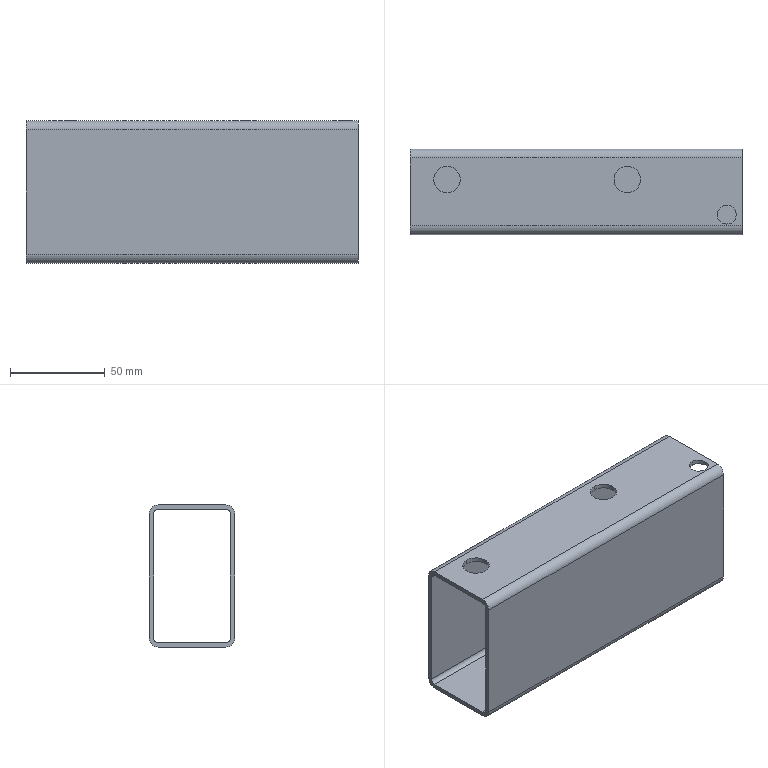Part | STEP file | [09] | 1 solid | 24 faces | box 175 x 45 x 75 mm | volume 89624 mm3 | cylinder 14 | plane 10 | commonest cylinder face diameters 4.6 x4 9.2 x4 14 x4 10 x2
STEP:
#1=CARTESIAN_POINT('',(167.,15.5,75.));
#2=VERTEX_POINT('',#1);
#3=CARTESIAN_POINT('',(167.,5.5,75.));
#4=VERTEX_POINT('',#3);
#5=CARTESIAN_POINT('',(167.,10.5,75.));
#6=DIRECTION('',(0.,0.,-1.));
#7=DIRECTION('',(0.,-1.,0.));
#8=AXIS2_PLACEMENT_3D('',#5,#6,#7);
#9=CIRCLE('',#8,5.);
#10=EDGE_CURVE('',#2,#4,#9,.T.);
#11=ORIENTED_EDGE('',*,*,#10,.F.);
#12=CARTESIAN_POINT('',(167.,15.5,72.7));
#13=VERTEX_POINT('',#12);
#14=CARTESIAN_POINT('',(167.,15.5,75.));
#15=DIRECTION('',(0.,0.,-1.));
#16=VECTOR('',#15,1000.);
#17=LINE('',#14,#16);
#18=EDGE_CURVE('',#2,#13,#17,.T.);
#19=ORIENTED_EDGE('',*,*,#18,.T.);
#20=CARTESIAN_POINT('',(167.,5.5,72.7));
#21=VERTEX_POINT('',#20);
#22=CARTESIAN_POINT('',(167.,10.5,72.7));
#23=DIRECTION('',(0.,0.,1.));
#24=DIRECTION('',(0.,1.,0.));
#25=AXIS2_PLACEMENT_3D('',#22,#23,#24);
#26=CIRCLE('',#25,5.);
#27=EDGE_CURVE('',#21,#13,#26,.T.);
#28=ORIENTED_EDGE('',*,*,#27,.F.);
#29=CARTESIAN_POINT('',(167.,5.5,75.));
#30=DIRECTION('',(0.,0.,-1.));
#31=VECTOR('',#30,1000.);
#32=LINE('',#29,#31);
#33=EDGE_CURVE('',#4,#21,#32,.T.);
#34=ORIENTED_EDGE('',*,*,#33,.F.);
#35=EDGE_LOOP('',(#11,#19,#28,#34));
#36=FACE_OUTER_BOUND('',#35,.T.);
#37=CARTESIAN_POINT('',(167.,10.5,75.));
#38=DIRECTION('',(0.,0.,-1.));
#39=DIRECTION('',(0.,-1.,0.));
#40=AXIS2_PLACEMENT_3D('',#37,#38,#39);
#41=CYLINDRICAL_SURFACE('',#40,5.);
#42=ADVANCED_FACE('',(#36),#41,.F.);
#43=CARTESIAN_POINT('',(114.5,36.,75.));
#44=VERTEX_POINT('',#43);
#45=CARTESIAN_POINT('',(114.5,22.,75.));
#46=VERTEX_POINT('',#45);
#47=CARTESIAN_POINT('',(114.5,29.,75.));
#48=DIRECTION('',(0.,0.,-1.));
#49=DIRECTION('',(0.,-1.,0.));
#50=AXIS2_PLACEMENT_3D('',#47,#48,#49);
#51=CIRCLE('',#50,7.);
#52=EDGE_CURVE('',#44,#46,#51,.T.);
#53=ORIENTED_EDGE('',*,*,#52,.F.);
#54=CARTESIAN_POINT('',(114.5,36.,72.7));
#55=VERTEX_POINT('',#54);
#56=CARTESIAN_POINT('',(114.5,36.,75.));
#57=DIRECTION('',(0.,0.,-1.));
#58=VECTOR('',#57,1000.);
#59=LINE('',#56,#58);
#60=EDGE_CURVE('',#44,#55,#59,.T.);
#61=ORIENTED_EDGE('',*,*,#60,.T.);
#62=CARTESIAN_POINT('',(114.5,22.,72.7));
#63=VERTEX_POINT('',#62);
#64=CARTESIAN_POINT('',(114.5,29.,72.7));
#65=DIRECTION('',(0.,0.,1.));
#66=DIRECTION('',(0.,1.,0.));
#67=AXIS2_PLACEMENT_3D('',#64,#65,#66);
#68=CIRCLE('',#67,7.);
#69=EDGE_CURVE('',#63,#55,#68,.T.);
#70=ORIENTED_EDGE('',*,*,#69,.F.);
#71=CARTESIAN_POINT('',(114.5,22.,75.));
#72=DIRECTION('',(0.,0.,-1.));
#73=VECTOR('',#72,1000.);
#74=LINE('',#71,#73);
#75=EDGE_CURVE('',#46,#63,#74,.T.);
#76=ORIENTED_EDGE('',*,*,#75,.F.);
#77=EDGE_LOOP('',(#53,#61,#70,#76));
#78=FACE_OUTER_BOUND('',#77,.T.);
#79=CARTESIAN_POINT('',(114.5,29.,75.));
#80=DIRECTION('',(0.,0.,-1.));
#81=DIRECTION('',(0.,-1.,0.));
#82=AXIS2_PLACEMENT_3D('',#79,#80,#81);
#83=CYLINDRICAL_SURFACE('',#82,7.);
#84=ADVANCED_FACE('',(#78),#83,.F.);
#85=CARTESIAN_POINT('',(19.5,36.,75.));
#86=VERTEX_POINT('',#85);
#87=CARTESIAN_POINT('',(19.5,22.,75.));
#88=VERTEX_POINT('',#87);
#89=CARTESIAN_POINT('',(19.5,29.,75.));
#90=DIRECTION('',(0.,0.,-1.));
#91=DIRECTION('',(0.,-1.,0.));
#92=AXIS2_PLACEMENT_3D('',#89,#90,#91);
#93=CIRCLE('',#92,7.);
#94=EDGE_CURVE('',#86,#88,#93,.T.);
#95=ORIENTED_EDGE('',*,*,#94,.F.);
#96=CARTESIAN_POINT('',(19.5,36.,72.7));
#97=VERTEX_POINT('',#96);
#98=CARTESIAN_POINT('',(19.5,36.,75.));
#99=DIRECTION('',(0.,0.,-1.));
#100=VECTOR('',#99,1000.);
#101=LINE('',#98,#100);
#102=EDGE_CURVE('',#86,#97,#101,.T.);
#103=ORIENTED_EDGE('',*,*,#102,.T.);
#104=CARTESIAN_POINT('',(19.5,22.,72.7));
#105=VERTEX_POINT('',#104);
#106=CARTESIAN_POINT('',(19.5,29.,72.7));
#107=DIRECTION('',(0.,0.,1.));
#108=DIRECTION('',(0.,1.,0.));
#109=AXIS2_PLACEMENT_3D('',#106,#107,#108);
#110=CIRCLE('',#109,7.);
#111=EDGE_CURVE('',#105,#97,#110,.T.);
#112=ORIENTED_EDGE('',*,*,#111,.F.);
#113=CARTESIAN_POINT('',(19.5,22.,75.));
#114=DIRECTION('',(0.,0.,-1.));
#115=VECTOR('',#114,1000.);
#116=LINE('',#113,#115);
#117=EDGE_CURVE('',#88,#105,#116,.T.);
#118=ORIENTED_EDGE('',*,*,#117,.F.);
#119=EDGE_LOOP('',(#95,#103,#112,#118));
#120=FACE_OUTER_BOUND('',#119,.T.);
#121=CARTESIAN_POINT('',(19.5,29.,75.));
#122=DIRECTION('',(0.,0.,-1.));
#123=DIRECTION('',(0.,-1.,0.));
#124=AXIS2_PLACEMENT_3D('',#121,#122,#123);
#125=CYLINDRICAL_SURFACE('',#124,7.);
#126=ADVANCED_FACE('',(#120),#125,.F.);
#127=CARTESIAN_POINT('',(0.,45.,70.4));
#128=VERTEX_POINT('',#127);
#129=CARTESIAN_POINT('',(0.,45.,4.6));
#130=VERTEX_POINT('',#129);
#131=CARTESIAN_POINT('',(0.,45.,70.4));
#132=DIRECTION('',(0.,0.,-1.));
#133=VECTOR('',#132,1000.);
#134=LINE('',#131,#133);
#135=EDGE_CURVE('',#128,#130,#134,.T.);
#136=ORIENTED_EDGE('',*,*,#135,.F.);
#137=CARTESIAN_POINT('',(175.,45.,70.4));
#138=VERTEX_POINT('',#137);
#139=CARTESIAN_POINT('',(175.,45.,70.4));
#140=DIRECTION('',(-1.,0.,0.));
#141=VECTOR('',#140,1000.);
#142=LINE('',#139,#141);
#143=EDGE_CURVE('',#138,#128,#142,.T.);
#144=ORIENTED_EDGE('',*,*,#143,.F.);
#145=CARTESIAN_POINT('',(175.,45.,4.6));
#146=VERTEX_POINT('',#145);
#147=CARTESIAN_POINT('',(175.,45.,70.4));
#148=DIRECTION('',(0.,0.,-1.));
#149=VECTOR('',#148,1000.);
#150=LINE('',#147,#149);
#151=EDGE_CURVE('',#138,#146,#150,.T.);
#152=ORIENTED_EDGE('',*,*,#151,.T.);
#153=CARTESIAN_POINT('',(175.,45.,4.6));
#154=DIRECTION('',(-1.,0.,0.));
#155=VECTOR('',#154,1000.);
#156=LINE('',#153,#155);
#157=EDGE_CURVE('',#146,#130,#156,.T.);
#158=ORIENTED_EDGE('',*,*,#157,.T.);
#159=EDGE_LOOP('',(#136,#144,#152,#158));
#160=FACE_OUTER_BOUND('',#159,.T.);
#161=CARTESIAN_POINT('',(175.,45.,70.4));
#162=DIRECTION('',(0.,1.,0.));
#163=DIRECTION('',(0.,0.,-1.));
#164=AXIS2_PLACEMENT_3D('',#161,#162,#163);
#165=PLANE('',#164);
#166=ADVANCED_FACE('',(#160),#165,.T.);
#167=CARTESIAN_POINT('',(0.,40.4,0.));
#168=VERTEX_POINT('',#167);
#169=CARTESIAN_POINT('',(0.,40.4,4.6));
#170=DIRECTION('',(-1.,0.,0.));
#171=DIRECTION('',(0.,1.,0.));
#172=AXIS2_PLACEMENT_3D('',#169,#170,#171);
#173=CIRCLE('',#172,4.6);
#174=EDGE_CURVE('',#130,#168,#173,.T.);
#175=ORIENTED_EDGE('',*,*,#174,.F.);
#176=ORIENTED_EDGE('',*,*,#157,.F.);
#177=CARTESIAN_POINT('',(175.,40.4,0.));
#178=VERTEX_POINT('',#177);
#179=CARTESIAN_POINT('',(175.,40.4,4.6));
#180=DIRECTION('',(-1.,0.,0.));
#181=DIRECTION('',(0.,1.,0.));
#182=AXIS2_PLACEMENT_3D('',#179,#180,#181);
#183=CIRCLE('',#182,4.6);
#184=EDGE_CURVE('',#146,#178,#183,.T.);
#185=ORIENTED_EDGE('',*,*,#184,.T.);
#186=CARTESIAN_POINT('',(175.,40.4,0.));
#187=DIRECTION('',(-1.,0.,0.));
#188=VECTOR('',#187,1000.);
#189=LINE('',#186,#188);
#190=EDGE_CURVE('',#178,#168,#189,.T.);
#191=ORIENTED_EDGE('',*,*,#190,.T.);
#192=EDGE_LOOP('',(#175,#176,#185,#191));
#193=FACE_OUTER_BOUND('',#192,.T.);
#194=CARTESIAN_POINT('',(175.,40.4,4.6));
#195=DIRECTION('',(-1.,0.,0.));
#196=DIRECTION('',(0.,1.,0.));
#197=AXIS2_PLACEMENT_3D('',#194,#195,#196);
#198=CYLINDRICAL_SURFACE('',#197,4.6);
#199=ADVANCED_FACE('',(#193),#198,.T.);
#200=CARTESIAN_POINT('',(0.,4.6,0.));
#201=VERTEX_POINT('',#200);
#202=CARTESIAN_POINT('',(0.,40.4,0.));
#203=DIRECTION('',(0.,-1.,0.));
#204=VECTOR('',#203,1000.);
#205=LINE('',#202,#204);
#206=EDGE_CURVE('',#168,#201,#205,.T.);
#207=ORIENTED_EDGE('',*,*,#206,.F.);
#208=ORIENTED_EDGE('',*,*,#190,.F.);
#209=CARTESIAN_POINT('',(175.,4.6,0.));
#210=VERTEX_POINT('',#209);
#211=CARTESIAN_POINT('',(175.,40.4,0.));
#212=DIRECTION('',(0.,-1.,0.));
#213=VECTOR('',#212,1000.);
#214=LINE('',#211,#213);
#215=EDGE_CURVE('',#178,#210,#214,.T.);
#216=ORIENTED_EDGE('',*,*,#215,.T.);
#217=CARTESIAN_POINT('',(175.,4.6,0.));
#218=DIRECTION('',(-1.,0.,0.));
#219=VECTOR('',#218,1000.);
#220=LINE('',#217,#219);
#221=EDGE_CURVE('',#210,#201,#220,.T.);
#222=ORIENTED_EDGE('',*,*,#221,.T.);
#223=EDGE_LOOP('',(#207,#208,#216,#222));
#224=FACE_OUTER_BOUND('',#223,.T.);
#225=CARTESIAN_POINT('',(175.,40.4,0.));
#226=DIRECTION('',(0.,0.,-1.));
#227=DIRECTION('',(0.,-1.,0.));
#228=AXIS2_PLACEMENT_3D('',#225,#226,#227);
#229=PLANE('',#228);
#230=ADVANCED_FACE('',(#224),#229,.T.);
#231=CARTESIAN_POINT('',(0.,0.,4.6));
#232=VERTEX_POINT('',#231);
#233=CARTESIAN_POINT('',(0.,4.6,4.6));
#234=DIRECTION('',(-1.,0.,0.));
#235=DIRECTION('',(0.,1.,0.));
#236=AXIS2_PLACEMENT_3D('',#233,#234,#235);
#237=CIRCLE('',#236,4.6);
#238=EDGE_CURVE('',#201,#232,#237,.T.);
#239=ORIENTED_EDGE('',*,*,#238,.F.);
#240=ORIENTED_EDGE('',*,*,#221,.F.);
#241=CARTESIAN_POINT('',(175.,0.,4.6));
#242=VERTEX_POINT('',#241);
#243=CARTESIAN_POINT('',(175.,4.6,4.6));
#244=DIRECTION('',(-1.,0.,0.));
#245=DIRECTION('',(0.,1.,0.));
#246=AXIS2_PLACEMENT_3D('',#243,#244,#245);
#247=CIRCLE('',#246,4.6);
#248=EDGE_CURVE('',#210,#242,#247,.T.);
#249=ORIENTED_EDGE('',*,*,#248,.T.);
#250=CARTESIAN_POINT('',(175.,0.,4.6));
#251=DIRECTION('',(-1.,0.,0.));
#252=VECTOR('',#251,1000.);
#253=LINE('',#250,#252);
#254=EDGE_CURVE('',#242,#232,#253,.T.);
#255=ORIENTED_EDGE('',*,*,#254,.T.);
#256=EDGE_LOOP('',(#239,#240,#249,#255));
#257=FACE_OUTER_BOUND('',#256,.T.);
#258=CARTESIAN_POINT('',(175.,4.6,4.6));
#259=DIRECTION('',(-1.,0.,0.));
#260=DIRECTION('',(0.,1.,0.));
#261=AXIS2_PLACEMENT_3D('',#258,#259,#260);
#262=CYLINDRICAL_SURFACE('',#261,4.6);
#263=ADVANCED_FACE('',(#257),#262,.T.);
#264=CARTESIAN_POINT('',(0.,0.,70.4));
#265=VERTEX_POINT('',#264);
#266=CARTESIAN_POINT('',(0.,0.,4.6));
#267=DIRECTION('',(0.,0.,1.));
#268=VECTOR('',#267,1000.);
#269=LINE('',#266,#268);
#270=EDGE_CURVE('',#232,#265,#269,.T.);
#271=ORIENTED_EDGE('',*,*,#270,.F.);
#272=ORIENTED_EDGE('',*,*,#254,.F.);
#273=CARTESIAN_POINT('',(175.,0.,70.4));
#274=VERTEX_POINT('',#273);
#275=CARTESIAN_POINT('',(175.,0.,4.6));
#276=DIRECTION('',(0.,0.,1.));
#277=VECTOR('',#276,1000.);
#278=LINE('',#275,#277);
#279=EDGE_CURVE('',#242,#274,#278,.T.);
#280=ORIENTED_EDGE('',*,*,#279,.T.);
#281=CARTESIAN_POINT('',(175.,0.,70.4));
#282=DIRECTION('',(-1.,0.,0.));
#283=VECTOR('',#282,1000.);
#284=LINE('',#281,#283);
#285=EDGE_CURVE('',#274,#265,#284,.T.);
#286=ORIENTED_EDGE('',*,*,#285,.T.);
#287=EDGE_LOOP('',(#271,#272,#280,#286));
#288=FACE_OUTER_BOUND('',#287,.T.);
#289=CARTESIAN_POINT('',(175.,0.,4.6));
#290=DIRECTION('',(0.,-1.,0.));
#291=DIRECTION('',(0.,0.,1.));
#292=AXIS2_PLACEMENT_3D('',#289,#290,#291);
#293=PLANE('',#292);
#294=ADVANCED_FACE('',(#288),#293,.T.);
#295=CARTESIAN_POINT('',(0.,4.6,75.));
#296=VERTEX_POINT('',#295);
#297=CARTESIAN_POINT('',(0.,4.6,70.4));
#298=DIRECTION('',(-1.,0.,0.));
#299=DIRECTION('',(0.,1.,0.));
#300=AXIS2_PLACEMENT_3D('',#297,#298,#299);
#301=CIRCLE('',#300,4.6);
#302=EDGE_CURVE('',#265,#296,#301,.T.);
#303=ORIENTED_EDGE('',*,*,#302,.F.);
#304=ORIENTED_EDGE('',*,*,#285,.F.);
#305=CARTESIAN_POINT('',(175.,4.6,75.));
#306=VERTEX_POINT('',#305);
#307=CARTESIAN_POINT('',(175.,4.6,70.4));
#308=DIRECTION('',(-1.,0.,0.));
#309=DIRECTION('',(0.,1.,0.));
#310=AXIS2_PLACEMENT_3D('',#307,#308,#309);
#311=CIRCLE('',#310,4.6);
#312=EDGE_CURVE('',#274,#306,#311,.T.);
#313=ORIENTED_EDGE('',*,*,#312,.T.);
#314=CARTESIAN_POINT('',(175.,4.6,75.));
#315=DIRECTION('',(-1.,0.,0.));
#316=VECTOR('',#315,1000.);
#317=LINE('',#314,#316);
#318=EDGE_CURVE('',#306,#296,#317,.T.);
#319=ORIENTED_EDGE('',*,*,#318,.T.);
#320=EDGE_LOOP('',(#303,#304,#313,#319));
#321=FACE_OUTER_BOUND('',#320,.T.);
#322=CARTESIAN_POINT('',(175.,4.6,70.4));
#323=DIRECTION('',(-1.,0.,0.));
#324=DIRECTION('',(0.,1.,0.));
#325=AXIS2_PLACEMENT_3D('',#322,#323,#324);
#326=CYLINDRICAL_SURFACE('',#325,4.6);
#327=ADVANCED_FACE('',(#321),#326,.T.);
#328=CARTESIAN_POINT('',(167.,10.5,75.));
#329=DIRECTION('',(0.,0.,-1.));
#330=DIRECTION('',(0.,-1.,0.));
#331=AXIS2_PLACEMENT_3D('',#328,#329,#330);
#332=CIRCLE('',#331,5.);
#333=EDGE_CURVE('',#4,#2,#332,.T.);
#334=ORIENTED_EDGE('',*,*,#333,.T.);
#335=ORIENTED_EDGE('',*,*,#10,.T.);
#336=EDGE_LOOP('',(#334,#335));
#337=FACE_BOUND('',#336,.T.);
#338=CARTESIAN_POINT('',(114.5,29.,75.));
#339=DIRECTION('',(0.,0.,-1.));
#340=DIRECTION('',(0.,-1.,0.));
#341=AXIS2_PLACEMENT_3D('',#338,#339,#340);
#342=CIRCLE('',#341,7.);
#343=EDGE_CURVE('',#46,#44,#342,.T.);
#344=ORIENTED_EDGE('',*,*,#343,.T.);
#345=ORIENTED_EDGE('',*,*,#52,.T.);
#346=EDGE_LOOP('',(#344,#345));
#347=FACE_BOUND('',#346,.T.);
#348=CARTESIAN_POINT('',(19.5,29.,75.));
#349=DIRECTION('',(0.,0.,-1.));
#350=DIRECTION('',(0.,-1.,0.));
#351=AXIS2_PLACEMENT_3D('',#348,#349,#350);
#352=CIRCLE('',#351,7.);
#353=EDGE_CURVE('',#88,#86,#352,.T.);
#354=ORIENTED_EDGE('',*,*,#353,.T.);
#355=ORIENTED_EDGE('',*,*,#94,.T.);
#356=EDGE_LOOP('',(#354,#355));
#357=FACE_BOUND('',#356,.T.);
#358=CARTESIAN_POINT('',(0.,40.4,75.));
#359=VERTEX_POINT('',#358);
#360=CARTESIAN_POINT('',(0.,4.6,75.));
#361=DIRECTION('',(0.,1.,0.));
#362=VECTOR('',#361,1000.);
#363=LINE('',#360,#362);
#364=EDGE_CURVE('',#296,#359,#363,.T.);
#365=ORIENTED_EDGE('',*,*,#364,.F.);
#366=ORIENTED_EDGE('',*,*,#318,.F.);
#367=CARTESIAN_POINT('',(175.,40.4,75.));
#368=VERTEX_POINT('',#367);
#369=CARTESIAN_POINT('',(175.,4.6,75.));
#370=DIRECTION('',(0.,1.,0.));
#371=VECTOR('',#370,1000.);
#372=LINE('',#369,#371);
#373=EDGE_CURVE('',#306,#368,#372,.T.);
#374=ORIENTED_EDGE('',*,*,#373,.T.);
#375=CARTESIAN_POINT('',(175.,40.4,75.));
#376=DIRECTION('',(-1.,0.,0.));
#377=VECTOR('',#376,1000.);
#378=LINE('',#375,#377);
#379=EDGE_CURVE('',#368,#359,#378,.T.);
#380=ORIENTED_EDGE('',*,*,#379,.T.);
#381=EDGE_LOOP('',(#365,#366,#374,#380));
#382=FACE_OUTER_BOUND('',#381,.T.);
#383=CARTESIAN_POINT('',(175.,4.6,75.));
#384=DIRECTION('',(0.,0.,1.));
#385=DIRECTION('',(1.,0.,0.));
#386=AXIS2_PLACEMENT_3D('',#383,#384,#385);
#387=PLANE('',#386);
#388=ADVANCED_FACE('',(#337,#347,#357,#382),#387,.T.);
#389=CARTESIAN_POINT('',(0.,40.4,70.4));
#390=DIRECTION('',(-1.,0.,0.));
#391=DIRECTION('',(0.,1.,0.));
#392=AXIS2_PLACEMENT_3D('',#389,#390,#391);
#393=CIRCLE('',#392,4.6);
#394=EDGE_CURVE('',#359,#128,#393,.T.);
#395=ORIENTED_EDGE('',*,*,#394,.F.);
#396=ORIENTED_EDGE('',*,*,#379,.F.);
#397=CARTESIAN_POINT('',(175.,40.4,70.4));
#398=DIRECTION('',(-1.,0.,0.));
#399=DIRECTION('',(0.,1.,0.));
#400=AXIS2_PLACEMENT_3D('',#397,#398,#399);
#401=CIRCLE('',#400,4.6);
#402=EDGE_CURVE('',#368,#138,#401,.T.);
#403=ORIENTED_EDGE('',*,*,#402,.T.);
#404=ORIENTED_EDGE('',*,*,#143,.T.);
#405=EDGE_LOOP('',(#395,#396,#403,#404));
#406=FACE_OUTER_BOUND('',#405,.T.);
#407=CARTESIAN_POINT('',(175.,40.4,70.4));
#408=DIRECTION('',(-1.,0.,0.));
#409=DIRECTION('',(0.,1.,0.));
#410=AXIS2_PLACEMENT_3D('',#407,#408,#409);
#411=CYLINDRICAL_SURFACE('',#410,4.6);
#412=ADVANCED_FACE('',(#406),#411,.T.);
#413=CARTESIAN_POINT('',(175.,4.6,72.7));
#414=VERTEX_POINT('',#413);
#415=CARTESIAN_POINT('',(175.,40.4,72.7));
#416=VERTEX_POINT('',#415);
#417=CARTESIAN_POINT('',(175.,4.6,72.7));
#418=DIRECTION('',(0.,1.,0.));
#419=VECTOR('',#418,1000.);
#420=LINE('',#417,#419);
#421=EDGE_CURVE('',#414,#416,#420,.T.);
#422=ORIENTED_EDGE('',*,*,#421,.T.);
#423=CARTESIAN_POINT('',(175.,42.7,70.4));
#424=VERTEX_POINT('',#423);
#425=CARTESIAN_POINT('',(175.,40.4,70.4));
#426=DIRECTION('',(-1.,0.,0.));
#427=DIRECTION('',(0.,0.,1.));
#428=AXIS2_PLACEMENT_3D('',#425,#426,#427);
#429=CIRCLE('',#428,2.3);
#430=EDGE_CURVE('',#416,#424,#429,.T.);
#431=ORIENTED_EDGE('',*,*,#430,.T.);
#432=CARTESIAN_POINT('',(175.,42.7,4.6));
#433=VERTEX_POINT('',#432);
#434=CARTESIAN_POINT('',(175.,42.7,70.4));
#435=DIRECTION('',(0.,0.,-1.));
#436=VECTOR('',#435,1000.);
#437=LINE('',#434,#436);
#438=EDGE_CURVE('',#424,#433,#437,.T.);
#439=ORIENTED_EDGE('',*,*,#438,.T.);
#440=CARTESIAN_POINT('',(175.,40.4,2.3));
#441=VERTEX_POINT('',#440);
#442=CARTESIAN_POINT('',(175.,40.4,4.6));
#443=DIRECTION('',(-1.,0.,0.));
#444=DIRECTION('',(0.,0.,1.));
#445=AXIS2_PLACEMENT_3D('',#442,#443,#444);
#446=CIRCLE('',#445,2.3);
#447=EDGE_CURVE('',#433,#441,#446,.T.);
#448=ORIENTED_EDGE('',*,*,#447,.T.);
#449=CARTESIAN_POINT('',(175.,4.6,2.3));
#450=VERTEX_POINT('',#449);
#451=CARTESIAN_POINT('',(175.,40.4,2.3));
#452=DIRECTION('',(0.,-1.,0.));
#453=VECTOR('',#452,1000.);
#454=LINE('',#451,#453);
#455=EDGE_CURVE('',#441,#450,#454,.T.);
#456=ORIENTED_EDGE('',*,*,#455,.T.);
#457=CARTESIAN_POINT('',(175.,2.3,4.6));
#458=VERTEX_POINT('',#457);
#459=CARTESIAN_POINT('',(175.,4.6,4.6));
#460=DIRECTION('',(-1.,0.,0.));
#461=DIRECTION('',(0.,0.,1.));
#462=AXIS2_PLACEMENT_3D('',#459,#460,#461);
#463=CIRCLE('',#462,2.3);
#464=EDGE_CURVE('',#450,#458,#463,.T.);
#465=ORIENTED_EDGE('',*,*,#464,.T.);
#466=CARTESIAN_POINT('',(175.,2.3,70.4));
#467=VERTEX_POINT('',#466);
#468=CARTESIAN_POINT('',(175.,2.3,4.6));
#469=DIRECTION('',(0.,0.,1.));
#470=VECTOR('',#469,1000.);
#471=LINE('',#468,#470);
#472=EDGE_CURVE('',#458,#467,#471,.T.);
#473=ORIENTED_EDGE('',*,*,#472,.T.);
#474=CARTESIAN_POINT('',(175.,4.6,70.4));
#475=DIRECTION('',(-1.,0.,0.));
#476=DIRECTION('',(0.,0.,1.));
#477=AXIS2_PLACEMENT_3D('',#474,#475,#476);
#478=CIRCLE('',#477,2.3);
#479=EDGE_CURVE('',#467,#414,#478,.T.);
#480=ORIENTED_EDGE('',*,*,#479,.T.);
#481=EDGE_LOOP('',(#422,#431,#439,#448,#456,#465,#473,#480));
#482=FACE_BOUND('',#481,.T.);
#483=ORIENTED_EDGE('',*,*,#151,.F.);
#484=ORIENTED_EDGE('',*,*,#402,.F.);
#485=ORIENTED_EDGE('',*,*,#373,.F.);
#486=ORIENTED_EDGE('',*,*,#312,.F.);
#487=ORIENTED_EDGE('',*,*,#279,.F.);
#488=ORIENTED_EDGE('',*,*,#248,.F.);
#489=ORIENTED_EDGE('',*,*,#215,.F.);
#490=ORIENTED_EDGE('',*,*,#184,.F.);
#491=EDGE_LOOP('',(#483,#484,#485,#486,#487,#488,#489,#490));
#492=FACE_OUTER_BOUND('',#491,.T.);
#493=CARTESIAN_POINT('',(175.,40.4,4.6));
#494=DIRECTION('',(-1.,0.,0.));
#495=DIRECTION('',(0.,1.,0.));
#496=AXIS2_PLACEMENT_3D('',#493,#494,#495);
#497=PLANE('',#496);
#498=ADVANCED_FACE('',(#482,#492),#497,.F.);
#499=CARTESIAN_POINT('',(0.,40.4,72.7));
#500=VERTEX_POINT('',#499);
#501=CARTESIAN_POINT('',(0.,42.7,70.4));
#502=VERTEX_POINT('',#501);
#503=CARTESIAN_POINT('',(0.,40.4,70.4));
#504=DIRECTION('',(-1.,0.,0.));
#505=DIRECTION('',(0.,0.,1.));
#506=AXIS2_PLACEMENT_3D('',#503,#504,#505);
#507=CIRCLE('',#506,2.3);
#508=EDGE_CURVE('',#500,#502,#507,.T.);
#509=ORIENTED_EDGE('',*,*,#508,.F.);
#510=CARTESIAN_POINT('',(0.,4.6,72.7));
#511=VERTEX_POINT('',#510);
#512=CARTESIAN_POINT('',(0.,4.6,72.7));
#513=DIRECTION('',(0.,1.,0.));
#514=VECTOR('',#513,1000.);
#515=LINE('',#512,#514);
#516=EDGE_CURVE('',#511,#500,#515,.T.);
#517=ORIENTED_EDGE('',*,*,#516,.F.);
#518=CARTESIAN_POINT('',(0.,2.3,70.4));
#519=VERTEX_POINT('',#518);
#520=CARTESIAN_POINT('',(0.,4.6,70.4));
#521=DIRECTION('',(-1.,0.,0.));
#522=DIRECTION('',(0.,0.,1.));
#523=AXIS2_PLACEMENT_3D('',#520,#521,#522);
#524=CIRCLE('',#523,2.3);
#525=EDGE_CURVE('',#519,#511,#524,.T.);
#526=ORIENTED_EDGE('',*,*,#525,.F.);
#527=CARTESIAN_POINT('',(0.,2.3,4.6));
#528=VERTEX_POINT('',#527);
#529=CARTESIAN_POINT('',(0.,2.3,4.6));
#530=DIRECTION('',(0.,0.,1.));
#531=VECTOR('',#530,1000.);
#532=LINE('',#529,#531);
#533=EDGE_CURVE('',#528,#519,#532,.T.);
#534=ORIENTED_EDGE('',*,*,#533,.F.);
#535=CARTESIAN_POINT('',(0.,4.6,2.3));
#536=VERTEX_POINT('',#535);
#537=CARTESIAN_POINT('',(0.,4.6,4.6));
#538=DIRECTION('',(-1.,0.,0.));
#539=DIRECTION('',(0.,0.,1.));
#540=AXIS2_PLACEMENT_3D('',#537,#538,#539);
#541=CIRCLE('',#540,2.3);
#542=EDGE_CURVE('',#536,#528,#541,.T.);
#543=ORIENTED_EDGE('',*,*,#542,.F.);
#544=CARTESIAN_POINT('',(0.,40.4,2.3));
#545=VERTEX_POINT('',#544);
#546=CARTESIAN_POINT('',(0.,40.4,2.3));
#547=DIRECTION('',(0.,-1.,0.));
#548=VECTOR('',#547,1000.);
#549=LINE('',#546,#548);
#550=EDGE_CURVE('',#545,#536,#549,.T.);
#551=ORIENTED_EDGE('',*,*,#550,.F.);
#552=CARTESIAN_POINT('',(0.,42.7,4.6));
#553=VERTEX_POINT('',#552);
#554=CARTESIAN_POINT('',(0.,40.4,4.6));
#555=DIRECTION('',(-1.,0.,0.));
#556=DIRECTION('',(0.,0.,1.));
#557=AXIS2_PLACEMENT_3D('',#554,#555,#556);
#558=CIRCLE('',#557,2.3);
#559=EDGE_CURVE('',#553,#545,#558,.T.);
#560=ORIENTED_EDGE('',*,*,#559,.F.);
#561=CARTESIAN_POINT('',(0.,42.7,70.4));
#562=DIRECTION('',(0.,0.,-1.));
#563=VECTOR('',#562,1000.);
#564=LINE('',#561,#563);
#565=EDGE_CURVE('',#502,#553,#564,.T.);
#566=ORIENTED_EDGE('',*,*,#565,.F.);
#567=EDGE_LOOP('',(#509,#517,#526,#534,#543,#551,#560,#566));
#568=FACE_BOUND('',#567,.T.);
#569=ORIENTED_EDGE('',*,*,#135,.T.);
#570=ORIENTED_EDGE('',*,*,#174,.T.);
#571=ORIENTED_EDGE('',*,*,#206,.T.);
#572=ORIENTED_EDGE('',*,*,#238,.T.);
#573=ORIENTED_EDGE('',*,*,#270,.T.);
#574=ORIENTED_EDGE('',*,*,#302,.T.);
#575=ORIENTED_EDGE('',*,*,#364,.T.);
#576=ORIENTED_EDGE('',*,*,#394,.T.);
#577=EDGE_LOOP('',(#569,#570,#571,#572,#573,#574,#575,#576));
#578=FACE_OUTER_BOUND('',#577,.T.);
#579=CARTESIAN_POINT('',(0.,40.4,4.6));
#580=DIRECTION('',(-1.,0.,0.));
#581=DIRECTION('',(0.,1.,0.));
#582=AXIS2_PLACEMENT_3D('',#579,#580,#581);
#583=PLANE('',#582);
#584=ADVANCED_FACE('',(#568,#578),#583,.T.);
#585=ORIENTED_EDGE('',*,*,#508,.T.);
#586=CARTESIAN_POINT('',(175.,42.7,70.4));
#587=DIRECTION('',(-1.,0.,0.));
#588=VECTOR('',#587,1000.);
#589=LINE('',#586,#588);
#590=EDGE_CURVE('',#424,#502,#589,.T.);
#591=ORIENTED_EDGE('',*,*,#590,.F.);
#592=ORIENTED_EDGE('',*,*,#430,.F.);
#593=CARTESIAN_POINT('',(175.,40.4,72.7));
#594=DIRECTION('',(-1.,0.,0.));
#595=VECTOR('',#594,1000.);
#596=LINE('',#593,#595);
#597=EDGE_CURVE('',#416,#500,#596,.T.);
#598=ORIENTED_EDGE('',*,*,#597,.T.);
#599=EDGE_LOOP('',(#585,#591,#592,#598));
#600=FACE_OUTER_BOUND('',#599,.T.);
#601=CARTESIAN_POINT('',(175.,40.4,70.4));
#602=DIRECTION('',(-1.,0.,0.));
#603=DIRECTION('',(0.,0.,1.));
#604=AXIS2_PLACEMENT_3D('',#601,#602,#603);
#605=CYLINDRICAL_SURFACE('',#604,2.3);
#606=ADVANCED_FACE('',(#600),#605,.F.);
#607=ORIENTED_EDGE('',*,*,#565,.T.);
#608=CARTESIAN_POINT('',(175.,42.7,4.6));
#609=DIRECTION('',(-1.,0.,0.));
#610=VECTOR('',#609,1000.);
#611=LINE('',#608,#610);
#612=EDGE_CURVE('',#433,#553,#611,.T.);
#613=ORIENTED_EDGE('',*,*,#612,.F.);
#614=ORIENTED_EDGE('',*,*,#438,.F.);
#615=ORIENTED_EDGE('',*,*,#590,.T.);
#616=EDGE_LOOP('',(#607,#613,#614,#615));
#617=FACE_OUTER_BOUND('',#616,.T.);
#618=CARTESIAN_POINT('',(175.,42.7,70.4));
#619=DIRECTION('',(0.,1.,0.));
#620=DIRECTION('',(-1.,0.,0.));
#621=AXIS2_PLACEMENT_3D('',#618,#619,#620);
#622=PLANE('',#621);
#623=ADVANCED_FACE('',(#617),#622,.F.);
#624=ORIENTED_EDGE('',*,*,#559,.T.);
#625=CARTESIAN_POINT('',(175.,40.4,2.3));
#626=DIRECTION('',(-1.,0.,0.));
#627=VECTOR('',#626,1000.);
#628=LINE('',#625,#627);
#629=EDGE_CURVE('',#441,#545,#628,.T.);
#630=ORIENTED_EDGE('',*,*,#629,.F.);
#631=ORIENTED_EDGE('',*,*,#447,.F.);
#632=ORIENTED_EDGE('',*,*,#612,.T.);
#633=EDGE_LOOP('',(#624,#630,#631,#632));
#634=FACE_OUTER_BOUND('',#633,.T.);
#635=CARTESIAN_POINT('',(175.,40.4,4.6));
#636=DIRECTION('',(-1.,0.,0.));
#637=DIRECTION('',(0.,0.,1.));
#638=AXIS2_PLACEMENT_3D('',#635,#636,#637);
#639=CYLINDRICAL_SURFACE('',#638,2.3);
#640=ADVANCED_FACE('',(#634),#639,.F.);
#641=ORIENTED_EDGE('',*,*,#550,.T.);
#642=CARTESIAN_POINT('',(175.,4.6,2.3));
#643=DIRECTION('',(-1.,0.,0.));
#644=VECTOR('',#643,1000.);
#645=LINE('',#642,#644);
#646=EDGE_CURVE('',#450,#536,#645,.T.);
#647=ORIENTED_EDGE('',*,*,#646,.F.);
#648=ORIENTED_EDGE('',*,*,#455,.F.);
#649=ORIENTED_EDGE('',*,*,#629,.T.);
#650=EDGE_LOOP('',(#641,#647,#648,#649));
#651=FACE_OUTER_BOUND('',#650,.T.);
#652=CARTESIAN_POINT('',(175.,40.4,2.3));
#653=DIRECTION('',(0.,0.,-1.));
#654=DIRECTION('',(-1.,0.,0.));
#655=AXIS2_PLACEMENT_3D('',#652,#653,#654);
#656=PLANE('',#655);
#657=ADVANCED_FACE('',(#651),#656,.F.);
#658=ORIENTED_EDGE('',*,*,#542,.T.);
#659=CARTESIAN_POINT('',(175.,2.3,4.6));
#660=DIRECTION('',(-1.,0.,0.));
#661=VECTOR('',#660,1000.);
#662=LINE('',#659,#661);
#663=EDGE_CURVE('',#458,#528,#662,.T.);
#664=ORIENTED_EDGE('',*,*,#663,.F.);
#665=ORIENTED_EDGE('',*,*,#464,.F.);
#666=ORIENTED_EDGE('',*,*,#646,.T.);
#667=EDGE_LOOP('',(#658,#664,#665,#666));
#668=FACE_OUTER_BOUND('',#667,.T.);
#669=CARTESIAN_POINT('',(175.,4.6,4.6));
#670=DIRECTION('',(-1.,0.,0.));
#671=DIRECTION('',(0.,0.,1.));
#672=AXIS2_PLACEMENT_3D('',#669,#670,#671);
#673=CYLINDRICAL_SURFACE('',#672,2.3);
#674=ADVANCED_FACE('',(#668),#673,.F.);
#675=ORIENTED_EDGE('',*,*,#533,.T.);
#676=CARTESIAN_POINT('',(175.,2.3,70.4));
#677=DIRECTION('',(-1.,0.,0.));
#678=VECTOR('',#677,1000.);
#679=LINE('',#676,#678);
#680=EDGE_CURVE('',#467,#519,#679,.T.);
#681=ORIENTED_EDGE('',*,*,#680,.F.);
#682=ORIENTED_EDGE('',*,*,#472,.F.);
#683=ORIENTED_EDGE('',*,*,#663,.T.);
#684=EDGE_LOOP('',(#675,#681,#682,#683));
#685=FACE_OUTER_BOUND('',#684,.T.);
#686=CARTESIAN_POINT('',(175.,2.3,4.6));
#687=DIRECTION('',(0.,-1.,0.));
#688=DIRECTION('',(0.,0.,1.));
#689=AXIS2_PLACEMENT_3D('',#686,#687,#688);
#690=PLANE('',#689);
#691=ADVANCED_FACE('',(#685),#690,.F.);
#692=ORIENTED_EDGE('',*,*,#525,.T.);
#693=CARTESIAN_POINT('',(175.,4.6,72.7));
#694=DIRECTION('',(-1.,0.,0.));
#695=VECTOR('',#694,1000.);
#696=LINE('',#693,#695);
#697=EDGE_CURVE('',#414,#511,#696,.T.);
#698=ORIENTED_EDGE('',*,*,#697,.F.);
#699=ORIENTED_EDGE('',*,*,#479,.F.);
#700=ORIENTED_EDGE('',*,*,#680,.T.);
#701=EDGE_LOOP('',(#692,#698,#699,#700));
#702=FACE_OUTER_BOUND('',#701,.T.);
#703=CARTESIAN_POINT('',(175.,4.6,70.4));
#704=DIRECTION('',(-1.,0.,0.));
#705=DIRECTION('',(0.,0.,1.));
#706=AXIS2_PLACEMENT_3D('',#703,#704,#705);
#707=CYLINDRICAL_SURFACE('',#706,2.3);
#708=ADVANCED_FACE('',(#702),#707,.F.);
#709=ORIENTED_EDGE('',*,*,#27,.T.);
#710=CARTESIAN_POINT('',(167.,10.5,72.7));
#711=DIRECTION('',(0.,0.,1.));
#712=DIRECTION('',(0.,1.,0.));
#713=AXIS2_PLACEMENT_3D('',#710,#711,#712);
#714=CIRCLE('',#713,5.);
#715=EDGE_CURVE('',#13,#21,#714,.T.);
#716=ORIENTED_EDGE('',*,*,#715,.T.);
#717=EDGE_LOOP('',(#709,#716));
#718=FACE_BOUND('',#717,.T.);
#719=ORIENTED_EDGE('',*,*,#69,.T.);
#720=CARTESIAN_POINT('',(114.5,29.,72.7));
#721=DIRECTION('',(0.,0.,1.));
#722=DIRECTION('',(0.,1.,0.));
#723=AXIS2_PLACEMENT_3D('',#720,#721,#722);
#724=CIRCLE('',#723,7.);
#725=EDGE_CURVE('',#55,#63,#724,.T.);
#726=ORIENTED_EDGE('',*,*,#725,.T.);
#727=EDGE_LOOP('',(#719,#726));
#728=FACE_BOUND('',#727,.T.);
#729=ORIENTED_EDGE('',*,*,#111,.T.);
#730=CARTESIAN_POINT('',(19.5,29.,72.7));
#731=DIRECTION('',(0.,0.,1.));
#732=DIRECTION('',(0.,1.,0.));
#733=AXIS2_PLACEMENT_3D('',#730,#731,#732);
#734=CIRCLE('',#733,7.);
#735=EDGE_CURVE('',#97,#105,#734,.T.);
#736=ORIENTED_EDGE('',*,*,#735,.T.);
#737=EDGE_LOOP('',(#729,#736));
#738=FACE_BOUND('',#737,.T.);
#739=ORIENTED_EDGE('',*,*,#516,.T.);
#740=ORIENTED_EDGE('',*,*,#597,.F.);
#741=ORIENTED_EDGE('',*,*,#421,.F.);
#742=ORIENTED_EDGE('',*,*,#697,.T.);
#743=EDGE_LOOP('',(#739,#740,#741,#742));
#744=FACE_OUTER_BOUND('',#743,.T.);
#745=CARTESIAN_POINT('',(175.,4.6,72.7));
#746=DIRECTION('',(0.,0.,1.));
#747=DIRECTION('',(0.,1.,0.));
#748=AXIS2_PLACEMENT_3D('',#745,#746,#747);
#749=PLANE('',#748);
#750=ADVANCED_FACE('',(#718,#728,#738,#744),#749,.F.);
#751=ORIENTED_EDGE('',*,*,#102,.F.);
#752=ORIENTED_EDGE('',*,*,#353,.F.);
#753=ORIENTED_EDGE('',*,*,#117,.T.);
#754=ORIENTED_EDGE('',*,*,#735,.F.);
#755=EDGE_LOOP('',(#751,#752,#753,#754));
#756=FACE_OUTER_BOUND('',#755,.T.);
#757=CARTESIAN_POINT('',(19.5,29.,75.));
#758=DIRECTION('',(0.,0.,-1.));
#759=DIRECTION('',(0.,-1.,0.));
#760=AXIS2_PLACEMENT_3D('',#757,#758,#759);
#761=CYLINDRICAL_SURFACE('',#760,7.);
#762=ADVANCED_FACE('',(#756),#761,.F.);
#763=ORIENTED_EDGE('',*,*,#60,.F.);
#764=ORIENTED_EDGE('',*,*,#343,.F.);
#765=ORIENTED_EDGE('',*,*,#75,.T.);
#766=ORIENTED_EDGE('',*,*,#725,.F.);
#767=EDGE_LOOP('',(#763,#764,#765,#766));
#768=FACE_OUTER_BOUND('',#767,.T.);
#769=CARTESIAN_POINT('',(114.5,29.,75.));
#770=DIRECTION('',(0.,0.,-1.));
#771=DIRECTION('',(0.,-1.,0.));
#772=AXIS2_PLACEMENT_3D('',#769,#770,#771);
#773=CYLINDRICAL_SURFACE('',#772,7.);
#774=ADVANCED_FACE('',(#768),#773,.F.);
#775=ORIENTED_EDGE('',*,*,#18,.F.);
#776=ORIENTED_EDGE('',*,*,#333,.F.);
#777=ORIENTED_EDGE('',*,*,#33,.T.);
#778=ORIENTED_EDGE('',*,*,#715,.F.);
#779=EDGE_LOOP('',(#775,#776,#777,#778));
#780=FACE_OUTER_BOUND('',#779,.T.);
#781=CARTESIAN_POINT('',(167.,10.5,75.));
#782=DIRECTION('',(0.,0.,-1.));
#783=DIRECTION('',(0.,-1.,0.));
#784=AXIS2_PLACEMENT_3D('',#781,#782,#783);
#785=CYLINDRICAL_SURFACE('',#784,5.);
#786=ADVANCED_FACE('',(#780),#785,.F.);
#787=CLOSED_SHELL('',(#42,#84,#126,#166,#199,#230,#263,#294,#327,#388,#412,#498,#584,#606,#623,#640,#657,#674,#691,#708,#750,#762,#774,#786));
#788=MANIFOLD_SOLID_BREP('',#787);
#789=CARTESIAN_POINT('',(0.,0.,0.));
#790=DIRECTION('',(0.,0.,1.));
#791=DIRECTION('',(1.,0.,0.));
#792=AXIS2_PLACEMENT_3D('',#789,#790,#791);
#793=(LENGTH_UNIT()NAMED_UNIT(*)SI_UNIT(.MILLI.,.METRE.));
#794=UNCERTAINTY_MEASURE_WITH_UNIT(LENGTH_MEASURE(0.00001),#793,'','');
#795=(NAMED_UNIT(*)PLANE_ANGLE_UNIT()SI_UNIT($,.RADIAN.));
#796=(NAMED_UNIT(*)SI_UNIT($,.STERADIAN.)SOLID_ANGLE_UNIT());
#797=(GEOMETRIC_REPRESENTATION_CONTEXT(3)GLOBAL_UNCERTAINTY_ASSIGNED_CONTEXT((#794))GLOBAL_UNIT_ASSIGNED_CONTEXT((#793,#795,#796))REPRESENTATION_CONTEXT('',''));
#798=ADVANCED_BREP_SHAPE_REPRESENTATION('',(#788,#792),#797);